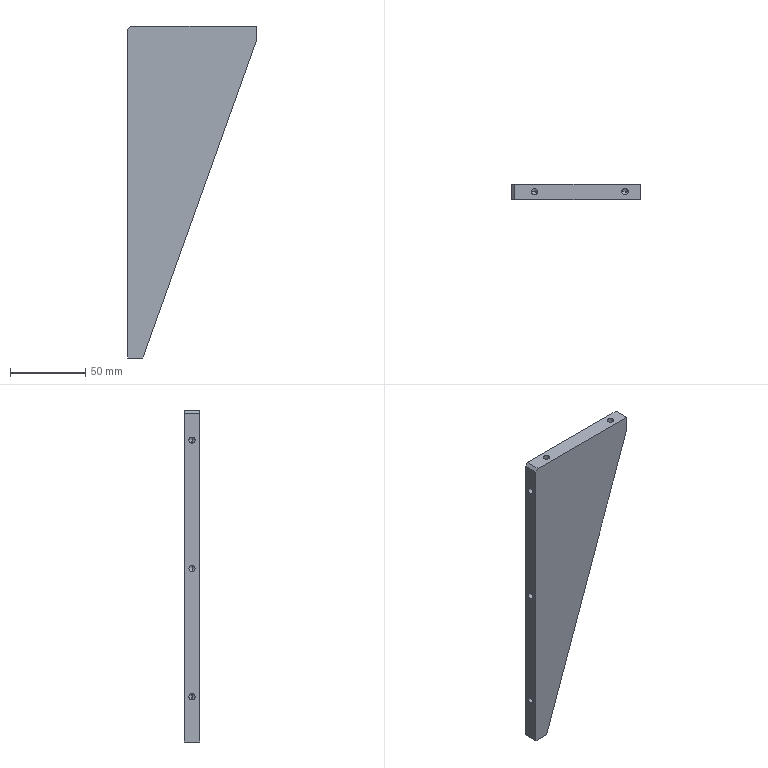Part | STEP file | PN_0057 | 1 solid | 28 faces | box 85 x 10 x 220 mm | volume 107342 mm3 | cylinder 10 | cone 10 | plane 8 | commonest cylinder face diameters 4.2 x10